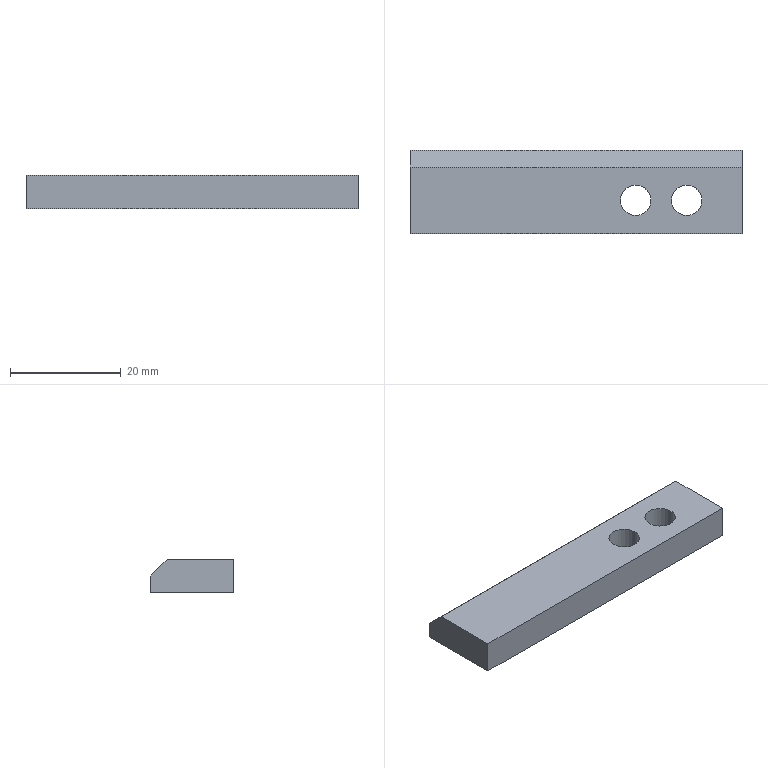Part | STEP file | cover plate 5 | 1 solid | 11 faces | box 60 x 15 x 6 mm | volume 4845 mm3 | plane 7 | cylinder 4 | commonest cylinder face diameters 5.5 x4
STEP:
#1=CARTESIAN_POINT('',(0.,0.,0.));
#2=DIRECTION('',(0.,0.,1.));
#3=DIRECTION('',(1.,0.,0.));
#4=AXIS2_PLACEMENT_3D('',#1,#2,#3);
#5=CARTESIAN_POINT('',(-28.562,0.,0.));
#6=VERTEX_POINT('',#5);
#7=CARTESIAN_POINT('',(-28.562,0.,6.));
#8=VERTEX_POINT('',#7);
#9=CARTESIAN_POINT('',(-28.562,0.,6.));
#10=DIRECTION('',(0.,0.,1.));
#11=VECTOR('',#10,1.);
#12=LINE('',#9,#11);
#13=CARTESIAN_POINT('',(-31.312,0.,6.));
#14=DIRECTION('',(0.,0.,1.));
#15=DIRECTION('',(1.,0.,0.));
#16=AXIS2_PLACEMENT_3D('',#13,#14,#15);
#17=CYLINDRICAL_SURFACE('',#16,2.75);
#18=CARTESIAN_POINT('',(6.283,0.));
#19=DIRECTION('',(0.,1.));
#20=VECTOR('',#19,1.);
#21=LINE('',#18,#20);
#22=(GEOMETRIC_REPRESENTATION_CONTEXT(2)PARAMETRIC_REPRESENTATION_CONTEXT()REPRESENTATION_CONTEXT('',''));
#23=DEFINITIONAL_REPRESENTATION('',(#21),#22);
#24=PCURVE('',#17,#23);
#25=CARTESIAN_POINT('',(-31.312,0.,6.));
#26=DIRECTION('',(0.,0.,1.));
#27=DIRECTION('',(1.,0.,0.));
#28=AXIS2_PLACEMENT_3D('',#25,#26,#27);
#29=CYLINDRICAL_SURFACE('',#28,2.75);
#30=CARTESIAN_POINT('',(0.,0.));
#31=DIRECTION('',(0.,1.));
#32=VECTOR('',#31,1.);
#33=LINE('',#30,#32);
#34=(GEOMETRIC_REPRESENTATION_CONTEXT(2)PARAMETRIC_REPRESENTATION_CONTEXT()REPRESENTATION_CONTEXT('',''));
#35=DEFINITIONAL_REPRESENTATION('',(#33),#34);
#36=PCURVE('',#29,#35);
#37=SURFACE_CURVE('',#12,(#24,#36),.PCURVE_S1.);
#38=EDGE_CURVE('',#6,#8,#37,.T.);
#39=ORIENTED_EDGE('',*,*,#38,.T.);
#40=CARTESIAN_POINT('',(-34.062,0.,6.));
#41=VERTEX_POINT('',#40);
#42=CARTESIAN_POINT('',(-31.312,0.,6.));
#43=DIRECTION('',(0.,0.,1.));
#44=DIRECTION('',(1.,0.,0.));
#45=AXIS2_PLACEMENT_3D('',#42,#43,#44);
#46=CIRCLE('',#45,2.75);
#47=CARTESIAN_POINT('',(0.,0.));
#48=DIRECTION('',(1.,0.));
#49=VECTOR('',#48,1.);
#50=LINE('',#47,#49);
#51=(GEOMETRIC_REPRESENTATION_CONTEXT(2)PARAMETRIC_REPRESENTATION_CONTEXT()REPRESENTATION_CONTEXT('',''));
#52=DEFINITIONAL_REPRESENTATION('',(#50),#51);
#53=PCURVE('',#17,#52);
#54=CARTESIAN_POINT('',(-72.112,-6.,6.));
#55=DIRECTION('',(0.,0.,1.));
#56=DIRECTION('',(1.,0.,0.));
#57=AXIS2_PLACEMENT_3D('',#54,#55,#56);
#58=PLANE('',#57);
#59=CARTESIAN_POINT('',(40.8,6.));
#60=DIRECTION('',(1.,0.));
#61=AXIS2_PLACEMENT_2D('',#59,#60);
#62=CIRCLE('',#61,2.75);
#63=(GEOMETRIC_REPRESENTATION_CONTEXT(2)PARAMETRIC_REPRESENTATION_CONTEXT()REPRESENTATION_CONTEXT('',''));
#64=DEFINITIONAL_REPRESENTATION('',(#62),#63);
#65=PCURVE('',#58,#64);
#66=SURFACE_CURVE('',#46,(#53,#65),.PCURVE_S1.);
#67=EDGE_CURVE('',#41,#8,#66,.T.);
#68=ORIENTED_EDGE('',*,*,#67,.F.);
#69=CARTESIAN_POINT('',(-34.062,0.,0.));
#70=VERTEX_POINT('',#69);
#71=CARTESIAN_POINT('',(-34.062,0.,6.));
#72=DIRECTION('',(0.,0.,1.));
#73=VECTOR('',#72,1.);
#74=LINE('',#71,#73);
#75=CARTESIAN_POINT('',(3.142,0.));
#76=DIRECTION('',(0.,1.));
#77=VECTOR('',#76,1.);
#78=LINE('',#75,#77);
#79=(GEOMETRIC_REPRESENTATION_CONTEXT(2)PARAMETRIC_REPRESENTATION_CONTEXT()REPRESENTATION_CONTEXT('',''));
#80=DEFINITIONAL_REPRESENTATION('',(#78),#79);
#81=PCURVE('',#17,#80);
#82=CARTESIAN_POINT('',(3.142,0.));
#83=DIRECTION('',(0.,1.));
#84=VECTOR('',#83,1.);
#85=LINE('',#82,#84);
#86=(GEOMETRIC_REPRESENTATION_CONTEXT(2)PARAMETRIC_REPRESENTATION_CONTEXT()REPRESENTATION_CONTEXT('',''));
#87=DEFINITIONAL_REPRESENTATION('',(#85),#86);
#88=PCURVE('',#29,#87);
#89=SURFACE_CURVE('',#74,(#81,#88),.PCURVE_S1.);
#90=EDGE_CURVE('',#70,#41,#89,.T.);
#91=ORIENTED_EDGE('',*,*,#90,.F.);
#92=CARTESIAN_POINT('',(-31.312,0.,0.));
#93=DIRECTION('',(0.,0.,1.));
#94=DIRECTION('',(1.,0.,0.));
#95=AXIS2_PLACEMENT_3D('',#92,#93,#94);
#96=CIRCLE('',#95,2.75);
#97=CARTESIAN_POINT('',(0.,-6.));
#98=DIRECTION('',(1.,0.));
#99=VECTOR('',#98,1.);
#100=LINE('',#97,#99);
#101=(GEOMETRIC_REPRESENTATION_CONTEXT(2)PARAMETRIC_REPRESENTATION_CONTEXT()REPRESENTATION_CONTEXT('',''));
#102=DEFINITIONAL_REPRESENTATION('',(#100),#101);
#103=PCURVE('',#17,#102);
#104=CARTESIAN_POINT('',(-72.112,-6.,0.));
#105=DIRECTION('',(0.,0.,1.));
#106=DIRECTION('',(1.,0.,0.));
#107=AXIS2_PLACEMENT_3D('',#104,#105,#106);
#108=PLANE('',#107);
#109=CARTESIAN_POINT('',(40.8,6.));
#110=DIRECTION('',(1.,0.));
#111=AXIS2_PLACEMENT_2D('',#109,#110);
#112=CIRCLE('',#111,2.75);
#113=(GEOMETRIC_REPRESENTATION_CONTEXT(2)PARAMETRIC_REPRESENTATION_CONTEXT()REPRESENTATION_CONTEXT('',''));
#114=DEFINITIONAL_REPRESENTATION('',(#112),#113);
#115=PCURVE('',#108,#114);
#116=SURFACE_CURVE('',#96,(#103,#115),.PCURVE_S1.);
#117=EDGE_CURVE('',#70,#6,#116,.T.);
#118=ORIENTED_EDGE('',*,*,#117,.T.);
#119=EDGE_LOOP('',(#39,#68,#91,#118));
#120=FACE_BOUND('',#119,.F.);
#121=ADVANCED_FACE('',(#120),#17,.F.);
#122=CARTESIAN_POINT('',(-19.362,0.,0.));
#123=VERTEX_POINT('',#122);
#124=CARTESIAN_POINT('',(-19.362,0.,6.));
#125=VERTEX_POINT('',#124);
#126=CARTESIAN_POINT('',(-19.362,0.,6.));
#127=DIRECTION('',(0.,0.,1.));
#128=VECTOR('',#127,1.);
#129=LINE('',#126,#128);
#130=CARTESIAN_POINT('',(-22.112,0.,6.));
#131=DIRECTION('',(0.,0.,1.));
#132=DIRECTION('',(1.,0.,0.));
#133=AXIS2_PLACEMENT_3D('',#130,#131,#132);
#134=CYLINDRICAL_SURFACE('',#133,2.75);
#135=CARTESIAN_POINT('',(6.283,0.));
#136=DIRECTION('',(0.,1.));
#137=VECTOR('',#136,1.);
#138=LINE('',#135,#137);
#139=(GEOMETRIC_REPRESENTATION_CONTEXT(2)PARAMETRIC_REPRESENTATION_CONTEXT()REPRESENTATION_CONTEXT('',''));
#140=DEFINITIONAL_REPRESENTATION('',(#138),#139);
#141=PCURVE('',#134,#140);
#142=CARTESIAN_POINT('',(-22.112,0.,6.));
#143=DIRECTION('',(0.,0.,1.));
#144=DIRECTION('',(1.,0.,0.));
#145=AXIS2_PLACEMENT_3D('',#142,#143,#144);
#146=CYLINDRICAL_SURFACE('',#145,2.75);
#147=CARTESIAN_POINT('',(0.,0.));
#148=DIRECTION('',(0.,1.));
#149=VECTOR('',#148,1.);
#150=LINE('',#147,#149);
#151=(GEOMETRIC_REPRESENTATION_CONTEXT(2)PARAMETRIC_REPRESENTATION_CONTEXT()REPRESENTATION_CONTEXT('',''));
#152=DEFINITIONAL_REPRESENTATION('',(#150),#151);
#153=PCURVE('',#146,#152);
#154=SURFACE_CURVE('',#129,(#141,#153),.PCURVE_S1.);
#155=EDGE_CURVE('',#123,#125,#154,.T.);
#156=ORIENTED_EDGE('',*,*,#155,.T.);
#157=CARTESIAN_POINT('',(-24.862,0.,6.));
#158=VERTEX_POINT('',#157);
#159=CARTESIAN_POINT('',(-22.112,0.,6.));
#160=DIRECTION('',(0.,0.,1.));
#161=DIRECTION('',(1.,0.,0.));
#162=AXIS2_PLACEMENT_3D('',#159,#160,#161);
#163=CIRCLE('',#162,2.75);
#164=CARTESIAN_POINT('',(0.,0.));
#165=DIRECTION('',(1.,0.));
#166=VECTOR('',#165,1.);
#167=LINE('',#164,#166);
#168=(GEOMETRIC_REPRESENTATION_CONTEXT(2)PARAMETRIC_REPRESENTATION_CONTEXT()REPRESENTATION_CONTEXT('',''));
#169=DEFINITIONAL_REPRESENTATION('',(#167),#168);
#170=PCURVE('',#134,#169);
#171=CARTESIAN_POINT('',(50.,6.));
#172=DIRECTION('',(1.,0.));
#173=AXIS2_PLACEMENT_2D('',#171,#172);
#174=CIRCLE('',#173,2.75);
#175=(GEOMETRIC_REPRESENTATION_CONTEXT(2)PARAMETRIC_REPRESENTATION_CONTEXT()REPRESENTATION_CONTEXT('',''));
#176=DEFINITIONAL_REPRESENTATION('',(#174),#175);
#177=PCURVE('',#58,#176);
#178=SURFACE_CURVE('',#163,(#170,#177),.PCURVE_S1.);
#179=EDGE_CURVE('',#158,#125,#178,.T.);
#180=ORIENTED_EDGE('',*,*,#179,.F.);
#181=CARTESIAN_POINT('',(-24.862,0.,0.));
#182=VERTEX_POINT('',#181);
#183=CARTESIAN_POINT('',(-24.862,0.,6.));
#184=DIRECTION('',(0.,0.,1.));
#185=VECTOR('',#184,1.);
#186=LINE('',#183,#185);
#187=CARTESIAN_POINT('',(3.142,0.));
#188=DIRECTION('',(0.,1.));
#189=VECTOR('',#188,1.);
#190=LINE('',#187,#189);
#191=(GEOMETRIC_REPRESENTATION_CONTEXT(2)PARAMETRIC_REPRESENTATION_CONTEXT()REPRESENTATION_CONTEXT('',''));
#192=DEFINITIONAL_REPRESENTATION('',(#190),#191);
#193=PCURVE('',#134,#192);
#194=CARTESIAN_POINT('',(3.142,0.));
#195=DIRECTION('',(0.,1.));
#196=VECTOR('',#195,1.);
#197=LINE('',#194,#196);
#198=(GEOMETRIC_REPRESENTATION_CONTEXT(2)PARAMETRIC_REPRESENTATION_CONTEXT()REPRESENTATION_CONTEXT('',''));
#199=DEFINITIONAL_REPRESENTATION('',(#197),#198);
#200=PCURVE('',#146,#199);
#201=SURFACE_CURVE('',#186,(#193,#200),.PCURVE_S1.);
#202=EDGE_CURVE('',#182,#158,#201,.T.);
#203=ORIENTED_EDGE('',*,*,#202,.F.);
#204=CARTESIAN_POINT('',(-22.112,0.,0.));
#205=DIRECTION('',(0.,0.,1.));
#206=DIRECTION('',(1.,0.,0.));
#207=AXIS2_PLACEMENT_3D('',#204,#205,#206);
#208=CIRCLE('',#207,2.75);
#209=CARTESIAN_POINT('',(0.,-6.));
#210=DIRECTION('',(1.,0.));
#211=VECTOR('',#210,1.);
#212=LINE('',#209,#211);
#213=(GEOMETRIC_REPRESENTATION_CONTEXT(2)PARAMETRIC_REPRESENTATION_CONTEXT()REPRESENTATION_CONTEXT('',''));
#214=DEFINITIONAL_REPRESENTATION('',(#212),#213);
#215=PCURVE('',#134,#214);
#216=CARTESIAN_POINT('',(50.,6.));
#217=DIRECTION('',(1.,0.));
#218=AXIS2_PLACEMENT_2D('',#216,#217);
#219=CIRCLE('',#218,2.75);
#220=(GEOMETRIC_REPRESENTATION_CONTEXT(2)PARAMETRIC_REPRESENTATION_CONTEXT()REPRESENTATION_CONTEXT('',''));
#221=DEFINITIONAL_REPRESENTATION('',(#219),#220);
#222=PCURVE('',#108,#221);
#223=SURFACE_CURVE('',#208,(#215,#222),.PCURVE_S1.);
#224=EDGE_CURVE('',#182,#123,#223,.T.);
#225=ORIENTED_EDGE('',*,*,#224,.T.);
#226=EDGE_LOOP('',(#156,#180,#203,#225));
#227=FACE_BOUND('',#226,.F.);
#228=ADVANCED_FACE('',(#227),#134,.F.);
#229=CARTESIAN_POINT('',(-72.112,6.,6.));
#230=VERTEX_POINT('',#229);
#231=CARTESIAN_POINT('',(-72.112,-6.,6.));
#232=VERTEX_POINT('',#231);
#233=CARTESIAN_POINT('',(-72.112,9.,6.));
#234=DIRECTION('',(0.,-1.,0.));
#235=VECTOR('',#234,1.);
#236=LINE('',#233,#235);
#237=CARTESIAN_POINT('',(-72.112,9.,6.));
#238=DIRECTION('',(1.,0.,0.));
#239=DIRECTION('',(0.,1.,0.));
#240=AXIS2_PLACEMENT_3D('',#237,#238,#239);
#241=PLANE('',#240);
#242=CARTESIAN_POINT('',(0.,0.));
#243=DIRECTION('',(-1.,0.));
#244=VECTOR('',#243,1.);
#245=LINE('',#242,#244);
#246=(GEOMETRIC_REPRESENTATION_CONTEXT(2)PARAMETRIC_REPRESENTATION_CONTEXT()REPRESENTATION_CONTEXT('',''));
#247=DEFINITIONAL_REPRESENTATION('',(#245),#246);
#248=PCURVE('',#241,#247);
#249=CARTESIAN_POINT('',(0.,15.));
#250=DIRECTION('',(0.,-1.));
#251=VECTOR('',#250,1.);
#252=LINE('',#249,#251);
#253=(GEOMETRIC_REPRESENTATION_CONTEXT(2)PARAMETRIC_REPRESENTATION_CONTEXT()REPRESENTATION_CONTEXT('',''));
#254=DEFINITIONAL_REPRESENTATION('',(#252),#253);
#255=PCURVE('',#58,#254);
#256=SURFACE_CURVE('',#236,(#248,#255),.PCURVE_S1.);
#257=EDGE_CURVE('',#230,#232,#256,.T.);
#258=ORIENTED_EDGE('',*,*,#257,.F.);
#259=CARTESIAN_POINT('',(-72.112,9.,3.));
#260=VERTEX_POINT('',#259);
#261=CARTESIAN_POINT('',(-72.112,6.,6.));
#262=DIRECTION('',(0.,0.7071,-0.7071));
#263=VECTOR('',#262,1.);
#264=LINE('',#261,#263);
#265=CARTESIAN_POINT('',(-3.,0.));
#266=DIRECTION('',(0.7071,-0.7071));
#267=VECTOR('',#266,1.);
#268=LINE('',#265,#267);
#269=(GEOMETRIC_REPRESENTATION_CONTEXT(2)PARAMETRIC_REPRESENTATION_CONTEXT()REPRESENTATION_CONTEXT('',''));
#270=DEFINITIONAL_REPRESENTATION('',(#268),#269);
#271=PCURVE('',#241,#270);
#272=CARTESIAN_POINT('',(-72.112,6.,6.));
#273=DIRECTION('',(0.,0.7071,0.7071));
#274=DIRECTION('',(0.,-0.7071,0.7071));
#275=AXIS2_PLACEMENT_3D('',#272,#273,#274);
#276=PLANE('',#275);
#277=CARTESIAN_POINT('',(0.,0.));
#278=DIRECTION('',(-1.,0.));
#279=VECTOR('',#278,1.);
#280=LINE('',#277,#279);
#281=(GEOMETRIC_REPRESENTATION_CONTEXT(2)PARAMETRIC_REPRESENTATION_CONTEXT()REPRESENTATION_CONTEXT('',''));
#282=DEFINITIONAL_REPRESENTATION('',(#280),#281);
#283=PCURVE('',#276,#282);
#284=SURFACE_CURVE('',#264,(#271,#283),.PCURVE_S1.);
#285=EDGE_CURVE('',#230,#260,#284,.T.);
#286=ORIENTED_EDGE('',*,*,#285,.T.);
#287=CARTESIAN_POINT('',(-72.112,9.,0.));
#288=VERTEX_POINT('',#287);
#289=CARTESIAN_POINT('',(-72.112,9.,6.));
#290=DIRECTION('',(0.,0.,-1.));
#291=VECTOR('',#290,1.);
#292=LINE('',#289,#291);
#293=CARTESIAN_POINT('',(0.,0.));
#294=DIRECTION('',(0.,-1.));
#295=VECTOR('',#294,1.);
#296=LINE('',#293,#295);
#297=(GEOMETRIC_REPRESENTATION_CONTEXT(2)PARAMETRIC_REPRESENTATION_CONTEXT()REPRESENTATION_CONTEXT('',''));
#298=DEFINITIONAL_REPRESENTATION('',(#296),#297);
#299=PCURVE('',#241,#298);
#300=CARTESIAN_POINT('',(-72.112,9.,6.));
#301=DIRECTION('',(0.,-1.,0.));
#302=DIRECTION('',(0.,0.,-1.));
#303=AXIS2_PLACEMENT_3D('',#300,#301,#302);
#304=PLANE('',#303);
#305=CARTESIAN_POINT('',(0.,0.));
#306=DIRECTION('',(1.,0.));
#307=VECTOR('',#306,1.);
#308=LINE('',#305,#307);
#309=(GEOMETRIC_REPRESENTATION_CONTEXT(2)PARAMETRIC_REPRESENTATION_CONTEXT()REPRESENTATION_CONTEXT('',''));
#310=DEFINITIONAL_REPRESENTATION('',(#308),#309);
#311=PCURVE('',#304,#310);
#312=SURFACE_CURVE('',#292,(#299,#311),.PCURVE_S1.);
#313=EDGE_CURVE('',#260,#288,#312,.T.);
#314=ORIENTED_EDGE('',*,*,#313,.T.);
#315=CARTESIAN_POINT('',(-72.112,-6.,0.));
#316=VERTEX_POINT('',#315);
#317=CARTESIAN_POINT('',(-72.112,9.,0.));
#318=DIRECTION('',(0.,-1.,0.));
#319=VECTOR('',#318,1.);
#320=LINE('',#317,#319);
#321=CARTESIAN_POINT('',(0.,-6.));
#322=DIRECTION('',(-1.,0.));
#323=VECTOR('',#322,1.);
#324=LINE('',#321,#323);
#325=(GEOMETRIC_REPRESENTATION_CONTEXT(2)PARAMETRIC_REPRESENTATION_CONTEXT()REPRESENTATION_CONTEXT('',''));
#326=DEFINITIONAL_REPRESENTATION('',(#324),#325);
#327=PCURVE('',#241,#326);
#328=CARTESIAN_POINT('',(0.,15.));
#329=DIRECTION('',(0.,-1.));
#330=VECTOR('',#329,1.);
#331=LINE('',#328,#330);
#332=(GEOMETRIC_REPRESENTATION_CONTEXT(2)PARAMETRIC_REPRESENTATION_CONTEXT()REPRESENTATION_CONTEXT('',''));
#333=DEFINITIONAL_REPRESENTATION('',(#331),#332);
#334=PCURVE('',#108,#333);
#335=SURFACE_CURVE('',#320,(#327,#334),.PCURVE_S1.);
#336=EDGE_CURVE('',#288,#316,#335,.T.);
#337=ORIENTED_EDGE('',*,*,#336,.T.);
#338=CARTESIAN_POINT('',(-72.112,-6.,6.));
#339=DIRECTION('',(0.,0.,-1.));
#340=VECTOR('',#339,1.);
#341=LINE('',#338,#340);
#342=CARTESIAN_POINT('',(-15.,0.));
#343=DIRECTION('',(0.,-1.));
#344=VECTOR('',#343,1.);
#345=LINE('',#342,#344);
#346=(GEOMETRIC_REPRESENTATION_CONTEXT(2)PARAMETRIC_REPRESENTATION_CONTEXT()REPRESENTATION_CONTEXT('',''));
#347=DEFINITIONAL_REPRESENTATION('',(#345),#346);
#348=PCURVE('',#241,#347);
#349=CARTESIAN_POINT('',(-72.112,-6.,6.));
#350=DIRECTION('',(0.,1.,0.));
#351=DIRECTION('',(-1.,0.,0.));
#352=AXIS2_PLACEMENT_3D('',#349,#350,#351);
#353=PLANE('',#352);
#354=CARTESIAN_POINT('',(0.,0.));
#355=DIRECTION('',(0.,-1.));
#356=VECTOR('',#355,1.);
#357=LINE('',#354,#356);
#358=(GEOMETRIC_REPRESENTATION_CONTEXT(2)PARAMETRIC_REPRESENTATION_CONTEXT()REPRESENTATION_CONTEXT('',''));
#359=DEFINITIONAL_REPRESENTATION('',(#357),#358);
#360=PCURVE('',#353,#359);
#361=SURFACE_CURVE('',#341,(#348,#360),.PCURVE_S1.);
#362=EDGE_CURVE('',#232,#316,#361,.T.);
#363=ORIENTED_EDGE('',*,*,#362,.F.);
#364=EDGE_LOOP('',(#258,#286,#314,#337,#363));
#365=FACE_BOUND('',#364,.T.);
#366=ADVANCED_FACE('',(#365),#241,.F.);
#367=CARTESIAN_POINT('',(-12.112,-6.,0.));
#368=VERTEX_POINT('',#367);
#369=CARTESIAN_POINT('',(-72.112,-6.,0.));
#370=DIRECTION('',(1.,0.,0.));
#371=VECTOR('',#370,1.);
#372=LINE('',#369,#371);
#373=CARTESIAN_POINT('',(0.,-6.));
#374=DIRECTION('',(-1.,0.));
#375=VECTOR('',#374,1.);
#376=LINE('',#373,#375);
#377=(GEOMETRIC_REPRESENTATION_CONTEXT(2)PARAMETRIC_REPRESENTATION_CONTEXT()REPRESENTATION_CONTEXT('',''));
#378=DEFINITIONAL_REPRESENTATION('',(#376),#377);
#379=PCURVE('',#353,#378);
#380=CARTESIAN_POINT('',(0.,0.));
#381=DIRECTION('',(1.,0.));
#382=VECTOR('',#381,1.);
#383=LINE('',#380,#382);
#384=(GEOMETRIC_REPRESENTATION_CONTEXT(2)PARAMETRIC_REPRESENTATION_CONTEXT()REPRESENTATION_CONTEXT('',''));
#385=DEFINITIONAL_REPRESENTATION('',(#383),#384);
#386=PCURVE('',#108,#385);
#387=SURFACE_CURVE('',#372,(#379,#386),.PCURVE_S1.);
#388=EDGE_CURVE('',#316,#368,#387,.T.);
#389=ORIENTED_EDGE('',*,*,#388,.T.);
#390=CARTESIAN_POINT('',(-12.112,-6.,6.));
#391=VERTEX_POINT('',#390);
#392=CARTESIAN_POINT('',(-12.112,-6.,6.));
#393=DIRECTION('',(0.,0.,-1.));
#394=VECTOR('',#393,1.);
#395=LINE('',#392,#394);
#396=CARTESIAN_POINT('',(-60.,0.));
#397=DIRECTION('',(0.,-1.));
#398=VECTOR('',#397,1.);
#399=LINE('',#396,#398);
#400=(GEOMETRIC_REPRESENTATION_CONTEXT(2)PARAMETRIC_REPRESENTATION_CONTEXT()REPRESENTATION_CONTEXT('',''));
#401=DEFINITIONAL_REPRESENTATION('',(#399),#400);
#402=PCURVE('',#353,#401);
#403=CARTESIAN_POINT('',(-12.112,9.,6.));
#404=DIRECTION('',(-1.,0.,0.));
#405=DIRECTION('',(0.,-1.,0.));
#406=AXIS2_PLACEMENT_3D('',#403,#404,#405);
#407=PLANE('',#406);
#408=CARTESIAN_POINT('',(15.,0.));
#409=DIRECTION('',(0.,-1.));
#410=VECTOR('',#409,1.);
#411=LINE('',#408,#410);
#412=(GEOMETRIC_REPRESENTATION_CONTEXT(2)PARAMETRIC_REPRESENTATION_CONTEXT()REPRESENTATION_CONTEXT('',''));
#413=DEFINITIONAL_REPRESENTATION('',(#411),#412);
#414=PCURVE('',#407,#413);
#415=SURFACE_CURVE('',#395,(#402,#414),.PCURVE_S1.);
#416=EDGE_CURVE('',#391,#368,#415,.T.);
#417=ORIENTED_EDGE('',*,*,#416,.F.);
#418=CARTESIAN_POINT('',(-72.112,-6.,6.));
#419=DIRECTION('',(1.,0.,0.));
#420=VECTOR('',#419,1.);
#421=LINE('',#418,#420);
#422=CARTESIAN_POINT('',(0.,0.));
#423=DIRECTION('',(-1.,0.));
#424=VECTOR('',#423,1.);
#425=LINE('',#422,#424);
#426=(GEOMETRIC_REPRESENTATION_CONTEXT(2)PARAMETRIC_REPRESENTATION_CONTEXT()REPRESENTATION_CONTEXT('',''));
#427=DEFINITIONAL_REPRESENTATION('',(#425),#426);
#428=PCURVE('',#353,#427);
#429=CARTESIAN_POINT('',(0.,0.));
#430=DIRECTION('',(1.,0.));
#431=VECTOR('',#430,1.);
#432=LINE('',#429,#431);
#433=(GEOMETRIC_REPRESENTATION_CONTEXT(2)PARAMETRIC_REPRESENTATION_CONTEXT()REPRESENTATION_CONTEXT('',''));
#434=DEFINITIONAL_REPRESENTATION('',(#432),#433);
#435=PCURVE('',#58,#434);
#436=SURFACE_CURVE('',#421,(#428,#435),.PCURVE_S1.);
#437=EDGE_CURVE('',#232,#391,#436,.T.);
#438=ORIENTED_EDGE('',*,*,#437,.F.);
#439=ORIENTED_EDGE('',*,*,#362,.T.);
#440=EDGE_LOOP('',(#389,#417,#438,#439));
#441=FACE_BOUND('',#440,.T.);
#442=ADVANCED_FACE('',(#441),#353,.F.);
#443=CARTESIAN_POINT('',(-12.112,9.,3.));
#444=VERTEX_POINT('',#443);
#445=CARTESIAN_POINT('',(-12.112,9.,0.));
#446=VERTEX_POINT('',#445);
#447=CARTESIAN_POINT('',(-12.112,9.,6.));
#448=DIRECTION('',(0.,0.,-1.));
#449=VECTOR('',#448,1.);
#450=LINE('',#447,#449);
#451=CARTESIAN_POINT('',(0.,0.));
#452=DIRECTION('',(0.,-1.));
#453=VECTOR('',#452,1.);
#454=LINE('',#451,#453);
#455=(GEOMETRIC_REPRESENTATION_CONTEXT(2)PARAMETRIC_REPRESENTATION_CONTEXT()REPRESENTATION_CONTEXT('',''));
#456=DEFINITIONAL_REPRESENTATION('',(#454),#455);
#457=PCURVE('',#407,#456);
#458=CARTESIAN_POINT('',(0.,60.));
#459=DIRECTION('',(1.,0.));
#460=VECTOR('',#459,1.);
#461=LINE('',#458,#460);
#462=(GEOMETRIC_REPRESENTATION_CONTEXT(2)PARAMETRIC_REPRESENTATION_CONTEXT()REPRESENTATION_CONTEXT('',''));
#463=DEFINITIONAL_REPRESENTATION('',(#461),#462);
#464=PCURVE('',#304,#463);
#465=SURFACE_CURVE('',#450,(#457,#464),.PCURVE_S1.);
#466=EDGE_CURVE('',#444,#446,#465,.T.);
#467=ORIENTED_EDGE('',*,*,#466,.F.);
#468=CARTESIAN_POINT('',(-12.112,6.,6.));
#469=VERTEX_POINT('',#468);
#470=CARTESIAN_POINT('',(-12.112,6.,6.));
#471=DIRECTION('',(0.,-0.7071,0.7071));
#472=VECTOR('',#471,1.);
#473=LINE('',#470,#472);
#474=CARTESIAN_POINT('',(3.,0.));
#475=DIRECTION('',(0.7071,0.7071));
#476=VECTOR('',#475,1.);
#477=LINE('',#474,#476);
#478=(GEOMETRIC_REPRESENTATION_CONTEXT(2)PARAMETRIC_REPRESENTATION_CONTEXT()REPRESENTATION_CONTEXT('',''));
#479=DEFINITIONAL_REPRESENTATION('',(#477),#478);
#480=PCURVE('',#407,#479);
#481=CARTESIAN_POINT('',(0.,60.));
#482=DIRECTION('',(1.,0.));
#483=VECTOR('',#482,1.);
#484=LINE('',#481,#483);
#485=(GEOMETRIC_REPRESENTATION_CONTEXT(2)PARAMETRIC_REPRESENTATION_CONTEXT()REPRESENTATION_CONTEXT('',''));
#486=DEFINITIONAL_REPRESENTATION('',(#484),#485);
#487=PCURVE('',#276,#486);
#488=SURFACE_CURVE('',#473,(#480,#487),.PCURVE_S1.);
#489=EDGE_CURVE('',#444,#469,#488,.T.);
#490=ORIENTED_EDGE('',*,*,#489,.T.);
#491=CARTESIAN_POINT('',(-12.112,9.,6.));
#492=DIRECTION('',(0.,1.,0.));
#493=VECTOR('',#492,1.);
#494=LINE('',#491,#493);
#495=CARTESIAN_POINT('',(0.,0.));
#496=DIRECTION('',(-1.,0.));
#497=VECTOR('',#496,1.);
#498=LINE('',#495,#497);
#499=(GEOMETRIC_REPRESENTATION_CONTEXT(2)PARAMETRIC_REPRESENTATION_CONTEXT()REPRESENTATION_CONTEXT('',''));
#500=DEFINITIONAL_REPRESENTATION('',(#498),#499);
#501=PCURVE('',#407,#500);
#502=CARTESIAN_POINT('',(60.,15.));
#503=DIRECTION('',(0.,1.));
#504=VECTOR('',#503,1.);
#505=LINE('',#502,#504);
#506=(GEOMETRIC_REPRESENTATION_CONTEXT(2)PARAMETRIC_REPRESENTATION_CONTEXT()REPRESENTATION_CONTEXT('',''));
#507=DEFINITIONAL_REPRESENTATION('',(#505),#506);
#508=PCURVE('',#58,#507);
#509=SURFACE_CURVE('',#494,(#501,#508),.PCURVE_S1.);
#510=EDGE_CURVE('',#391,#469,#509,.T.);
#511=ORIENTED_EDGE('',*,*,#510,.F.);
#512=ORIENTED_EDGE('',*,*,#416,.T.);
#513=CARTESIAN_POINT('',(-12.112,9.,0.));
#514=DIRECTION('',(0.,1.,0.));
#515=VECTOR('',#514,1.);
#516=LINE('',#513,#515);
#517=CARTESIAN_POINT('',(0.,-6.));
#518=DIRECTION('',(-1.,0.));
#519=VECTOR('',#518,1.);
#520=LINE('',#517,#519);
#521=(GEOMETRIC_REPRESENTATION_CONTEXT(2)PARAMETRIC_REPRESENTATION_CONTEXT()REPRESENTATION_CONTEXT('',''));
#522=DEFINITIONAL_REPRESENTATION('',(#520),#521);
#523=PCURVE('',#407,#522);
#524=CARTESIAN_POINT('',(60.,15.));
#525=DIRECTION('',(0.,1.));
#526=VECTOR('',#525,1.);
#527=LINE('',#524,#526);
#528=(GEOMETRIC_REPRESENTATION_CONTEXT(2)PARAMETRIC_REPRESENTATION_CONTEXT()REPRESENTATION_CONTEXT('',''));
#529=DEFINITIONAL_REPRESENTATION('',(#527),#528);
#530=PCURVE('',#108,#529);
#531=SURFACE_CURVE('',#516,(#523,#530),.PCURVE_S1.);
#532=EDGE_CURVE('',#368,#446,#531,.T.);
#533=ORIENTED_EDGE('',*,*,#532,.T.);
#534=EDGE_LOOP('',(#467,#490,#511,#512,#533));
#535=FACE_BOUND('',#534,.T.);
#536=ADVANCED_FACE('',(#535),#407,.F.);
#537=ORIENTED_EDGE('',*,*,#313,.F.);
#538=CARTESIAN_POINT('',(-12.112,9.,3.));
#539=DIRECTION('',(1.,0.,0.));
#540=VECTOR('',#539,1.);
#541=LINE('',#538,#540);
#542=CARTESIAN_POINT('',(3.,60.));
#543=DIRECTION('',(0.,1.));
#544=VECTOR('',#543,1.);
#545=LINE('',#542,#544);
#546=(GEOMETRIC_REPRESENTATION_CONTEXT(2)PARAMETRIC_REPRESENTATION_CONTEXT()REPRESENTATION_CONTEXT('',''));
#547=DEFINITIONAL_REPRESENTATION('',(#545),#546);
#548=PCURVE('',#304,#547);
#549=CARTESIAN_POINT('',(-4.243,60.));
#550=DIRECTION('',(0.,1.));
#551=VECTOR('',#550,1.);
#552=LINE('',#549,#551);
#553=(GEOMETRIC_REPRESENTATION_CONTEXT(2)PARAMETRIC_REPRESENTATION_CONTEXT()REPRESENTATION_CONTEXT('',''));
#554=DEFINITIONAL_REPRESENTATION('',(#552),#553);
#555=PCURVE('',#276,#554);
#556=SURFACE_CURVE('',#541,(#548,#555),.PCURVE_S1.);
#557=EDGE_CURVE('',#260,#444,#556,.T.);
#558=ORIENTED_EDGE('',*,*,#557,.T.);
#559=ORIENTED_EDGE('',*,*,#466,.T.);
#560=CARTESIAN_POINT('',(-72.112,9.,0.));
#561=DIRECTION('',(-1.,0.,0.));
#562=VECTOR('',#561,1.);
#563=LINE('',#560,#562);
#564=CARTESIAN_POINT('',(6.,0.));
#565=DIRECTION('',(0.,-1.));
#566=VECTOR('',#565,1.);
#567=LINE('',#564,#566);
#568=(GEOMETRIC_REPRESENTATION_CONTEXT(2)PARAMETRIC_REPRESENTATION_CONTEXT()REPRESENTATION_CONTEXT('',''));
#569=DEFINITIONAL_REPRESENTATION('',(#567),#568);
#570=PCURVE('',#304,#569);
#571=CARTESIAN_POINT('',(0.,15.));
#572=DIRECTION('',(-1.,0.));
#573=VECTOR('',#572,1.);
#574=LINE('',#571,#573);
#575=(GEOMETRIC_REPRESENTATION_CONTEXT(2)PARAMETRIC_REPRESENTATION_CONTEXT()REPRESENTATION_CONTEXT('',''));
#576=DEFINITIONAL_REPRESENTATION('',(#574),#575);
#577=PCURVE('',#108,#576);
#578=SURFACE_CURVE('',#563,(#570,#577),.PCURVE_S1.);
#579=EDGE_CURVE('',#446,#288,#578,.T.);
#580=ORIENTED_EDGE('',*,*,#579,.T.);
#581=EDGE_LOOP('',(#537,#558,#559,#580));
#582=FACE_BOUND('',#581,.T.);
#583=ADVANCED_FACE('',(#582),#304,.F.);
#584=CARTESIAN_POINT('',(-31.312,0.,6.));
#585=DIRECTION('',(0.,0.,1.));
#586=DIRECTION('',(1.,0.,0.));
#587=AXIS2_PLACEMENT_3D('',#584,#585,#586);
#588=CIRCLE('',#587,2.75);
#589=CARTESIAN_POINT('',(40.8,6.));
#590=DIRECTION('',(1.,0.));
#591=AXIS2_PLACEMENT_2D('',#589,#590);
#592=CIRCLE('',#591,2.75);
#593=(GEOMETRIC_REPRESENTATION_CONTEXT(2)PARAMETRIC_REPRESENTATION_CONTEXT()REPRESENTATION_CONTEXT('',''));
#594=DEFINITIONAL_REPRESENTATION('',(#592),#593);
#595=PCURVE('',#58,#594);
#596=CARTESIAN_POINT('',(0.,0.));
#597=DIRECTION('',(1.,0.));
#598=VECTOR('',#597,1.);
#599=LINE('',#596,#598);
#600=(GEOMETRIC_REPRESENTATION_CONTEXT(2)PARAMETRIC_REPRESENTATION_CONTEXT()REPRESENTATION_CONTEXT('',''));
#601=DEFINITIONAL_REPRESENTATION('',(#599),#600);
#602=PCURVE('',#29,#601);
#603=SURFACE_CURVE('',#588,(#595,#602),.PCURVE_S1.);
#604=EDGE_CURVE('',#8,#41,#603,.T.);
#605=ORIENTED_EDGE('',*,*,#604,.F.);
#606=ORIENTED_EDGE('',*,*,#67,.F.);
#607=EDGE_LOOP('',(#605,#606));
#608=FACE_BOUND('',#607,.T.);
#609=CARTESIAN_POINT('',(-22.112,0.,6.));
#610=DIRECTION('',(0.,0.,1.));
#611=DIRECTION('',(1.,0.,0.));
#612=AXIS2_PLACEMENT_3D('',#609,#610,#611);
#613=CIRCLE('',#612,2.75);
#614=CARTESIAN_POINT('',(50.,6.));
#615=DIRECTION('',(1.,0.));
#616=AXIS2_PLACEMENT_2D('',#614,#615);
#617=CIRCLE('',#616,2.75);
#618=(GEOMETRIC_REPRESENTATION_CONTEXT(2)PARAMETRIC_REPRESENTATION_CONTEXT()REPRESENTATION_CONTEXT('',''));
#619=DEFINITIONAL_REPRESENTATION('',(#617),#618);
#620=PCURVE('',#58,#619);
#621=CARTESIAN_POINT('',(0.,0.));
#622=DIRECTION('',(1.,0.));
#623=VECTOR('',#622,1.);
#624=LINE('',#621,#623);
#625=(GEOMETRIC_REPRESENTATION_CONTEXT(2)PARAMETRIC_REPRESENTATION_CONTEXT()REPRESENTATION_CONTEXT('',''));
#626=DEFINITIONAL_REPRESENTATION('',(#624),#625);
#627=PCURVE('',#146,#626);
#628=SURFACE_CURVE('',#613,(#620,#627),.PCURVE_S1.);
#629=EDGE_CURVE('',#125,#158,#628,.T.);
#630=ORIENTED_EDGE('',*,*,#629,.F.);
#631=ORIENTED_EDGE('',*,*,#179,.F.);
#632=EDGE_LOOP('',(#630,#631));
#633=FACE_BOUND('',#632,.T.);
#634=ORIENTED_EDGE('',*,*,#510,.T.);
#635=CARTESIAN_POINT('',(-72.112,6.,6.));
#636=DIRECTION('',(-1.,0.,0.));
#637=VECTOR('',#636,1.);
#638=LINE('',#635,#637);
#639=CARTESIAN_POINT('',(0.,12.));
#640=DIRECTION('',(-1.,0.));
#641=VECTOR('',#640,1.);
#642=LINE('',#639,#641);
#643=(GEOMETRIC_REPRESENTATION_CONTEXT(2)PARAMETRIC_REPRESENTATION_CONTEXT()REPRESENTATION_CONTEXT('',''));
#644=DEFINITIONAL_REPRESENTATION('',(#642),#643);
#645=PCURVE('',#58,#644);
#646=CARTESIAN_POINT('',(0.,0.));
#647=DIRECTION('',(0.,-1.));
#648=VECTOR('',#647,1.);
#649=LINE('',#646,#648);
#650=(GEOMETRIC_REPRESENTATION_CONTEXT(2)PARAMETRIC_REPRESENTATION_CONTEXT()REPRESENTATION_CONTEXT('',''));
#651=DEFINITIONAL_REPRESENTATION('',(#649),#650);
#652=PCURVE('',#276,#651);
#653=SURFACE_CURVE('',#638,(#645,#652),.PCURVE_S1.);
#654=EDGE_CURVE('',#469,#230,#653,.T.);
#655=ORIENTED_EDGE('',*,*,#654,.T.);
#656=ORIENTED_EDGE('',*,*,#257,.T.);
#657=ORIENTED_EDGE('',*,*,#437,.T.);
#658=EDGE_LOOP('',(#634,#655,#656,#657));
#659=FACE_BOUND('',#658,.T.);
#660=ADVANCED_FACE('',(#608,#633,#659),#58,.T.);
#661=CARTESIAN_POINT('',(-31.312,0.,0.));
#662=DIRECTION('',(0.,0.,1.));
#663=DIRECTION('',(1.,0.,0.));
#664=AXIS2_PLACEMENT_3D('',#661,#662,#663);
#665=CIRCLE('',#664,2.75);
#666=CARTESIAN_POINT('',(40.8,6.));
#667=DIRECTION('',(1.,0.));
#668=AXIS2_PLACEMENT_2D('',#666,#667);
#669=CIRCLE('',#668,2.75);
#670=(GEOMETRIC_REPRESENTATION_CONTEXT(2)PARAMETRIC_REPRESENTATION_CONTEXT()REPRESENTATION_CONTEXT('',''));
#671=DEFINITIONAL_REPRESENTATION('',(#669),#670);
#672=PCURVE('',#108,#671);
#673=CARTESIAN_POINT('',(0.,-6.));
#674=DIRECTION('',(1.,0.));
#675=VECTOR('',#674,1.);
#676=LINE('',#673,#675);
#677=(GEOMETRIC_REPRESENTATION_CONTEXT(2)PARAMETRIC_REPRESENTATION_CONTEXT()REPRESENTATION_CONTEXT('',''));
#678=DEFINITIONAL_REPRESENTATION('',(#676),#677);
#679=PCURVE('',#29,#678);
#680=SURFACE_CURVE('',#665,(#672,#679),.PCURVE_S1.);
#681=EDGE_CURVE('',#6,#70,#680,.T.);
#682=ORIENTED_EDGE('',*,*,#681,.T.);
#683=ORIENTED_EDGE('',*,*,#117,.T.);
#684=EDGE_LOOP('',(#682,#683));
#685=FACE_BOUND('',#684,.T.);
#686=CARTESIAN_POINT('',(-22.112,0.,0.));
#687=DIRECTION('',(0.,0.,1.));
#688=DIRECTION('',(1.,0.,0.));
#689=AXIS2_PLACEMENT_3D('',#686,#687,#688);
#690=CIRCLE('',#689,2.75);
#691=CARTESIAN_POINT('',(50.,6.));
#692=DIRECTION('',(1.,0.));
#693=AXIS2_PLACEMENT_2D('',#691,#692);
#694=CIRCLE('',#693,2.75);
#695=(GEOMETRIC_REPRESENTATION_CONTEXT(2)PARAMETRIC_REPRESENTATION_CONTEXT()REPRESENTATION_CONTEXT('',''));
#696=DEFINITIONAL_REPRESENTATION('',(#694),#695);
#697=PCURVE('',#108,#696);
#698=CARTESIAN_POINT('',(0.,-6.));
#699=DIRECTION('',(1.,0.));
#700=VECTOR('',#699,1.);
#701=LINE('',#698,#700);
#702=(GEOMETRIC_REPRESENTATION_CONTEXT(2)PARAMETRIC_REPRESENTATION_CONTEXT()REPRESENTATION_CONTEXT('',''));
#703=DEFINITIONAL_REPRESENTATION('',(#701),#702);
#704=PCURVE('',#146,#703);
#705=SURFACE_CURVE('',#690,(#697,#704),.PCURVE_S1.);
#706=EDGE_CURVE('',#123,#182,#705,.T.);
#707=ORIENTED_EDGE('',*,*,#706,.T.);
#708=ORIENTED_EDGE('',*,*,#224,.T.);
#709=EDGE_LOOP('',(#707,#708));
#710=FACE_BOUND('',#709,.T.);
#711=ORIENTED_EDGE('',*,*,#336,.F.);
#712=ORIENTED_EDGE('',*,*,#579,.F.);
#713=ORIENTED_EDGE('',*,*,#532,.F.);
#714=ORIENTED_EDGE('',*,*,#388,.F.);
#715=EDGE_LOOP('',(#711,#712,#713,#714));
#716=FACE_BOUND('',#715,.T.);
#717=ADVANCED_FACE('',(#685,#710,#716),#108,.F.);
#718=ORIENTED_EDGE('',*,*,#489,.F.);
#719=ORIENTED_EDGE('',*,*,#557,.F.);
#720=ORIENTED_EDGE('',*,*,#285,.F.);
#721=ORIENTED_EDGE('',*,*,#654,.F.);
#722=EDGE_LOOP('',(#718,#719,#720,#721));
#723=FACE_BOUND('',#722,.T.);
#724=ADVANCED_FACE('',(#723),#276,.T.);
#725=ORIENTED_EDGE('',*,*,#629,.F.);
#726=ORIENTED_EDGE('',*,*,#155,.F.);
#727=ORIENTED_EDGE('',*,*,#706,.T.);
#728=ORIENTED_EDGE('',*,*,#202,.T.);
#729=EDGE_LOOP('',(#725,#726,#727,#728));
#730=FACE_BOUND('',#729,.F.);
#731=ADVANCED_FACE('',(#730),#146,.F.);
#732=ORIENTED_EDGE('',*,*,#604,.F.);
#733=ORIENTED_EDGE('',*,*,#38,.F.);
#734=ORIENTED_EDGE('',*,*,#681,.T.);
#735=ORIENTED_EDGE('',*,*,#90,.T.);
#736=EDGE_LOOP('',(#732,#733,#734,#735));
#737=FACE_BOUND('',#736,.F.);
#738=ADVANCED_FACE('',(#737),#29,.F.);
#739=CLOSED_SHELL('',(#121,#228,#366,#442,#536,#583,#660,#717,#724,#731,#738));
#740=MANIFOLD_SOLID_BREP('',#739);
#741=(LENGTH_UNIT()NAMED_UNIT(*)SI_UNIT(.MILLI.,.METRE.));
#742=UNCERTAINTY_MEASURE_WITH_UNIT(LENGTH_MEASURE(0.0000001),#741,'','');
#743=(NAMED_UNIT(*)PLANE_ANGLE_UNIT()SI_UNIT($,.RADIAN.));
#744=(NAMED_UNIT(*)SI_UNIT($,.STERADIAN.)SOLID_ANGLE_UNIT());
#745=(GEOMETRIC_REPRESENTATION_CONTEXT(3)GLOBAL_UNCERTAINTY_ASSIGNED_CONTEXT((#742))GLOBAL_UNIT_ASSIGNED_CONTEXT((#741,#743,#744))REPRESENTATION_CONTEXT('',''));
#746=ADVANCED_BREP_SHAPE_REPRESENTATION('',(#4,#740),#745);